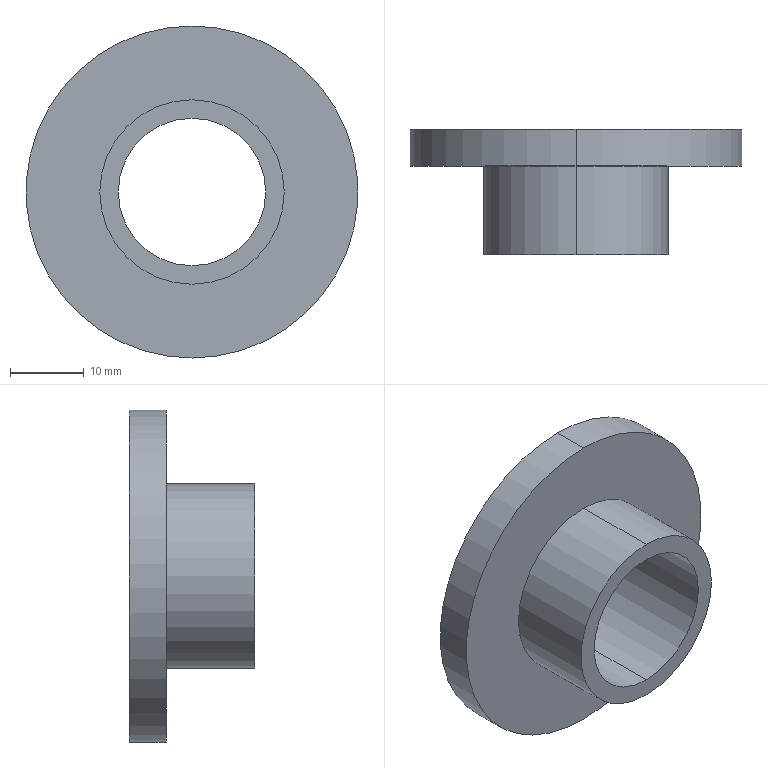Part | SolidWorks | features ICE 1, Revolution 1 | 1 solid | 9 faces | box 45 x 17 x 45 mm | volume 8502 mm3 | cylinder 6 | plane 3 | commonest cylinder face diameters 20 x2 25 x2 45 x2
STEP:
#1=CARTESIAN_POINT('',(0.,0.,-10.));
#2=VERTEX_POINT('',#1);
#3=CARTESIAN_POINT('',(0.,0.,10.));
#4=VERTEX_POINT('',#3);
#5=CARTESIAN_POINT('',(0.,0.,0.));
#6=DIRECTION('',(0.,1.,0.));
#7=DIRECTION('',(0.,0.,1.));
#8=AXIS2_PLACEMENT_3D('',#5,#6,#7);
#9=CIRCLE('',#8,10.);
#10=EDGE_CURVE('',#2,#4,#9,.T.);
#11=ORIENTED_EDGE('',*,*,#10,.T.);
#12=CARTESIAN_POINT('',(0.,-17.,10.));
#13=VERTEX_POINT('',#12);
#14=CARTESIAN_POINT('',(0.,9.,10.));
#15=DIRECTION('',(0.,-1.,0.));
#16=VECTOR('',#15,1000.);
#17=LINE('',#14,#16);
#18=EDGE_CURVE('',#4,#13,#17,.T.);
#19=ORIENTED_EDGE('',*,*,#18,.T.);
#20=CARTESIAN_POINT('',(0.,-17.,-10.));
#21=VERTEX_POINT('',#20);
#22=CARTESIAN_POINT('',(0.,-17.,0.));
#23=DIRECTION('',(0.,-1.,0.));
#24=DIRECTION('',(0.,0.,-1.));
#25=AXIS2_PLACEMENT_3D('',#22,#23,#24);
#26=CIRCLE('',#25,10.);
#27=EDGE_CURVE('',#13,#21,#26,.T.);
#28=ORIENTED_EDGE('',*,*,#27,.T.);
#29=CARTESIAN_POINT('',(0.,9.,-10.));
#30=DIRECTION('',(0.,-1.,0.));
#31=VECTOR('',#30,1000.);
#32=LINE('',#29,#31);
#33=EDGE_CURVE('',#2,#21,#32,.T.);
#34=ORIENTED_EDGE('',*,*,#33,.F.);
#35=EDGE_LOOP('',(#11,#19,#28,#34));
#36=FACE_OUTER_BOUND('',#35,.T.);
#37=CARTESIAN_POINT('',(0.,9.,0.));
#38=DIRECTION('',(0.,-1.,0.));
#39=DIRECTION('',(0.,0.,-1.));
#40=AXIS2_PLACEMENT_3D('',#37,#38,#39);
#41=CYLINDRICAL_SURFACE('',#40,10.);
#42=ADVANCED_FACE('',(#36),#41,.F.);
#43=CARTESIAN_POINT('',(0.,-5.,-12.5));
#44=VERTEX_POINT('',#43);
#45=CARTESIAN_POINT('',(0.,-5.,12.5));
#46=VERTEX_POINT('',#45);
#47=CARTESIAN_POINT('',(0.,-5.,0.));
#48=DIRECTION('',(0.,-1.,0.));
#49=DIRECTION('',(0.,0.,-1.));
#50=AXIS2_PLACEMENT_3D('',#47,#48,#49);
#51=CIRCLE('',#50,12.5);
#52=EDGE_CURVE('',#44,#46,#51,.T.);
#53=ORIENTED_EDGE('',*,*,#52,.T.);
#54=CARTESIAN_POINT('',(0.,-17.,12.5));
#55=VERTEX_POINT('',#54);
#56=CARTESIAN_POINT('',(0.,0.,12.5));
#57=DIRECTION('',(0.,-1.,0.));
#58=VECTOR('',#57,1000.);
#59=LINE('',#56,#58);
#60=EDGE_CURVE('',#46,#55,#59,.T.);
#61=ORIENTED_EDGE('',*,*,#60,.T.);
#62=CARTESIAN_POINT('',(0.,-17.,-12.5));
#63=VERTEX_POINT('',#62);
#64=CARTESIAN_POINT('',(0.,-17.,0.));
#65=DIRECTION('',(0.,-1.,0.));
#66=DIRECTION('',(0.,0.,-1.));
#67=AXIS2_PLACEMENT_3D('',#64,#65,#66);
#68=CIRCLE('',#67,12.5);
#69=EDGE_CURVE('',#63,#55,#68,.T.);
#70=ORIENTED_EDGE('',*,*,#69,.F.);
#71=CARTESIAN_POINT('',(0.,0.,-12.5));
#72=DIRECTION('',(0.,-1.,0.));
#73=VECTOR('',#72,1000.);
#74=LINE('',#71,#73);
#75=EDGE_CURVE('',#44,#63,#74,.T.);
#76=ORIENTED_EDGE('',*,*,#75,.F.);
#77=EDGE_LOOP('',(#53,#61,#70,#76));
#78=FACE_OUTER_BOUND('',#77,.T.);
#79=CARTESIAN_POINT('',(0.,0.,0.));
#80=DIRECTION('',(0.,-1.,0.));
#81=DIRECTION('',(0.,0.,-1.));
#82=AXIS2_PLACEMENT_3D('',#79,#80,#81);
#83=CYLINDRICAL_SURFACE('',#82,12.5);
#84=ADVANCED_FACE('',(#78),#83,.T.);
#85=CARTESIAN_POINT('',(0.,0.,-22.5));
#86=VERTEX_POINT('',#85);
#87=CARTESIAN_POINT('',(0.,0.,22.5));
#88=VERTEX_POINT('',#87);
#89=CARTESIAN_POINT('',(0.,0.,0.));
#90=DIRECTION('',(0.,-1.,0.));
#91=DIRECTION('',(0.,0.,-1.));
#92=AXIS2_PLACEMENT_3D('',#89,#90,#91);
#93=CIRCLE('',#92,22.5);
#94=EDGE_CURVE('',#86,#88,#93,.T.);
#95=ORIENTED_EDGE('',*,*,#94,.T.);
#96=CARTESIAN_POINT('',(0.,-5.,22.5));
#97=VERTEX_POINT('',#96);
#98=CARTESIAN_POINT('',(0.,0.,22.5));
#99=DIRECTION('',(0.,-1.,0.));
#100=VECTOR('',#99,1000.);
#101=LINE('',#98,#100);
#102=EDGE_CURVE('',#88,#97,#101,.T.);
#103=ORIENTED_EDGE('',*,*,#102,.T.);
#104=CARTESIAN_POINT('',(0.,-5.,-22.5));
#105=VERTEX_POINT('',#104);
#106=CARTESIAN_POINT('',(0.,-5.,0.));
#107=DIRECTION('',(0.,-1.,0.));
#108=DIRECTION('',(0.,0.,-1.));
#109=AXIS2_PLACEMENT_3D('',#106,#107,#108);
#110=CIRCLE('',#109,22.5);
#111=EDGE_CURVE('',#105,#97,#110,.T.);
#112=ORIENTED_EDGE('',*,*,#111,.F.);
#113=CARTESIAN_POINT('',(0.,0.,-22.5));
#114=DIRECTION('',(0.,-1.,0.));
#115=VECTOR('',#114,1000.);
#116=LINE('',#113,#115);
#117=EDGE_CURVE('',#86,#105,#116,.T.);
#118=ORIENTED_EDGE('',*,*,#117,.F.);
#119=EDGE_LOOP('',(#95,#103,#112,#118));
#120=FACE_OUTER_BOUND('',#119,.T.);
#121=CARTESIAN_POINT('',(0.,0.,0.));
#122=DIRECTION('',(0.,-1.,0.));
#123=DIRECTION('',(0.,0.,-1.));
#124=AXIS2_PLACEMENT_3D('',#121,#122,#123);
#125=CYLINDRICAL_SURFACE('',#124,22.5);
#126=ADVANCED_FACE('',(#120),#125,.T.);
#127=ORIENTED_EDGE('',*,*,#10,.F.);
#128=CARTESIAN_POINT('',(0.,0.,0.));
#129=DIRECTION('',(0.,1.,0.));
#130=DIRECTION('',(0.,0.,1.));
#131=AXIS2_PLACEMENT_3D('',#128,#129,#130);
#132=CIRCLE('',#131,10.);
#133=EDGE_CURVE('',#4,#2,#132,.T.);
#134=ORIENTED_EDGE('',*,*,#133,.F.);
#135=EDGE_LOOP('',(#127,#134));
#136=FACE_BOUND('',#135,.T.);
#137=ORIENTED_EDGE('',*,*,#94,.F.);
#138=CARTESIAN_POINT('',(0.,0.,0.));
#139=DIRECTION('',(0.,-1.,0.));
#140=DIRECTION('',(0.,0.,-1.));
#141=AXIS2_PLACEMENT_3D('',#138,#139,#140);
#142=CIRCLE('',#141,22.5);
#143=EDGE_CURVE('',#88,#86,#142,.T.);
#144=ORIENTED_EDGE('',*,*,#143,.F.);
#145=EDGE_LOOP('',(#137,#144));
#146=FACE_OUTER_BOUND('',#145,.T.);
#147=CARTESIAN_POINT('',(0.,0.,0.));
#148=DIRECTION('',(0.,1.,0.));
#149=DIRECTION('',(0.,0.,1.));
#150=AXIS2_PLACEMENT_3D('',#147,#148,#149);
#151=PLANE('',#150);
#152=ADVANCED_FACE('',(#136,#146),#151,.T.);
#153=ORIENTED_EDGE('',*,*,#102,.F.);
#154=ORIENTED_EDGE('',*,*,#143,.T.);
#155=ORIENTED_EDGE('',*,*,#117,.T.);
#156=CARTESIAN_POINT('',(0.,-5.,0.));
#157=DIRECTION('',(0.,-1.,0.));
#158=DIRECTION('',(0.,0.,-1.));
#159=AXIS2_PLACEMENT_3D('',#156,#157,#158);
#160=CIRCLE('',#159,22.5);
#161=EDGE_CURVE('',#97,#105,#160,.T.);
#162=ORIENTED_EDGE('',*,*,#161,.F.);
#163=EDGE_LOOP('',(#153,#154,#155,#162));
#164=FACE_OUTER_BOUND('',#163,.T.);
#165=CARTESIAN_POINT('',(0.,0.,0.));
#166=DIRECTION('',(0.,-1.,0.));
#167=DIRECTION('',(0.,0.,-1.));
#168=AXIS2_PLACEMENT_3D('',#165,#166,#167);
#169=CYLINDRICAL_SURFACE('',#168,22.5);
#170=ADVANCED_FACE('',(#164),#169,.T.);
#171=ORIENTED_EDGE('',*,*,#111,.T.);
#172=ORIENTED_EDGE('',*,*,#161,.T.);
#173=EDGE_LOOP('',(#171,#172));
#174=FACE_OUTER_BOUND('',#173,.T.);
#175=ORIENTED_EDGE('',*,*,#52,.F.);
#176=CARTESIAN_POINT('',(0.,-5.,0.));
#177=DIRECTION('',(0.,-1.,0.));
#178=DIRECTION('',(0.,0.,-1.));
#179=AXIS2_PLACEMENT_3D('',#176,#177,#178);
#180=CIRCLE('',#179,12.5);
#181=EDGE_CURVE('',#46,#44,#180,.T.);
#182=ORIENTED_EDGE('',*,*,#181,.F.);
#183=EDGE_LOOP('',(#175,#182));
#184=FACE_BOUND('',#183,.T.);
#185=CARTESIAN_POINT('',(22.5,-5.,0.));
#186=DIRECTION('',(0.,-1.,0.));
#187=DIRECTION('',(0.,0.,-1.));
#188=AXIS2_PLACEMENT_3D('',#185,#186,#187);
#189=PLANE('',#188);
#190=ADVANCED_FACE('',(#174,#184),#189,.T.);
#191=ORIENTED_EDGE('',*,*,#60,.F.);
#192=ORIENTED_EDGE('',*,*,#181,.T.);
#193=ORIENTED_EDGE('',*,*,#75,.T.);
#194=CARTESIAN_POINT('',(0.,-17.,0.));
#195=DIRECTION('',(0.,-1.,0.));
#196=DIRECTION('',(0.,0.,-1.));
#197=AXIS2_PLACEMENT_3D('',#194,#195,#196);
#198=CIRCLE('',#197,12.5);
#199=EDGE_CURVE('',#55,#63,#198,.T.);
#200=ORIENTED_EDGE('',*,*,#199,.F.);
#201=EDGE_LOOP('',(#191,#192,#193,#200));
#202=FACE_OUTER_BOUND('',#201,.T.);
#203=CARTESIAN_POINT('',(0.,0.,0.));
#204=DIRECTION('',(0.,-1.,0.));
#205=DIRECTION('',(0.,0.,-1.));
#206=AXIS2_PLACEMENT_3D('',#203,#204,#205);
#207=CYLINDRICAL_SURFACE('',#206,12.5);
#208=ADVANCED_FACE('',(#202),#207,.T.);
#209=CARTESIAN_POINT('',(0.,-17.,0.));
#210=DIRECTION('',(0.,-1.,0.));
#211=DIRECTION('',(0.,0.,-1.));
#212=AXIS2_PLACEMENT_3D('',#209,#210,#211);
#213=CIRCLE('',#212,10.);
#214=EDGE_CURVE('',#21,#13,#213,.T.);
#215=ORIENTED_EDGE('',*,*,#214,.F.);
#216=ORIENTED_EDGE('',*,*,#27,.F.);
#217=EDGE_LOOP('',(#215,#216));
#218=FACE_BOUND('',#217,.T.);
#219=ORIENTED_EDGE('',*,*,#69,.T.);
#220=ORIENTED_EDGE('',*,*,#199,.T.);
#221=EDGE_LOOP('',(#219,#220));
#222=FACE_OUTER_BOUND('',#221,.T.);
#223=CARTESIAN_POINT('',(12.5,-17.,0.));
#224=DIRECTION('',(0.,-1.,0.));
#225=DIRECTION('',(0.,0.,-1.));
#226=AXIS2_PLACEMENT_3D('',#223,#224,#225);
#227=PLANE('',#226);
#228=ADVANCED_FACE('',(#218,#222),#227,.T.);
#229=ORIENTED_EDGE('',*,*,#18,.F.);
#230=ORIENTED_EDGE('',*,*,#133,.T.);
#231=ORIENTED_EDGE('',*,*,#33,.T.);
#232=ORIENTED_EDGE('',*,*,#214,.T.);
#233=EDGE_LOOP('',(#229,#230,#231,#232));
#234=FACE_OUTER_BOUND('',#233,.T.);
#235=CARTESIAN_POINT('',(0.,9.,0.));
#236=DIRECTION('',(0.,-1.,0.));
#237=DIRECTION('',(0.,0.,-1.));
#238=AXIS2_PLACEMENT_3D('',#235,#236,#237);
#239=CYLINDRICAL_SURFACE('',#238,10.);
#240=ADVANCED_FACE('',(#234),#239,.F.);
#241=CLOSED_SHELL('',(#42,#84,#126,#152,#170,#190,#208,#228,#240));
#242=MANIFOLD_SOLID_BREP('',#241);
#243=CARTESIAN_POINT('',(0.,0.,0.));
#244=DIRECTION('',(0.,0.,1.));
#245=DIRECTION('',(1.,0.,0.));
#246=AXIS2_PLACEMENT_3D('',#243,#244,#245);
#247=(LENGTH_UNIT()NAMED_UNIT(*)SI_UNIT(.MILLI.,.METRE.));
#248=UNCERTAINTY_MEASURE_WITH_UNIT(LENGTH_MEASURE(0.00001),#247,'','');
#249=(NAMED_UNIT(*)PLANE_ANGLE_UNIT()SI_UNIT($,.RADIAN.));
#250=(NAMED_UNIT(*)SI_UNIT($,.STERADIAN.)SOLID_ANGLE_UNIT());
#251=(GEOMETRIC_REPRESENTATION_CONTEXT(3)GLOBAL_UNCERTAINTY_ASSIGNED_CONTEXT((#248))GLOBAL_UNIT_ASSIGNED_CONTEXT((#247,#249,#250))REPRESENTATION_CONTEXT('',''));
#252=ADVANCED_BREP_SHAPE_REPRESENTATION('',(#242,#246),#251);